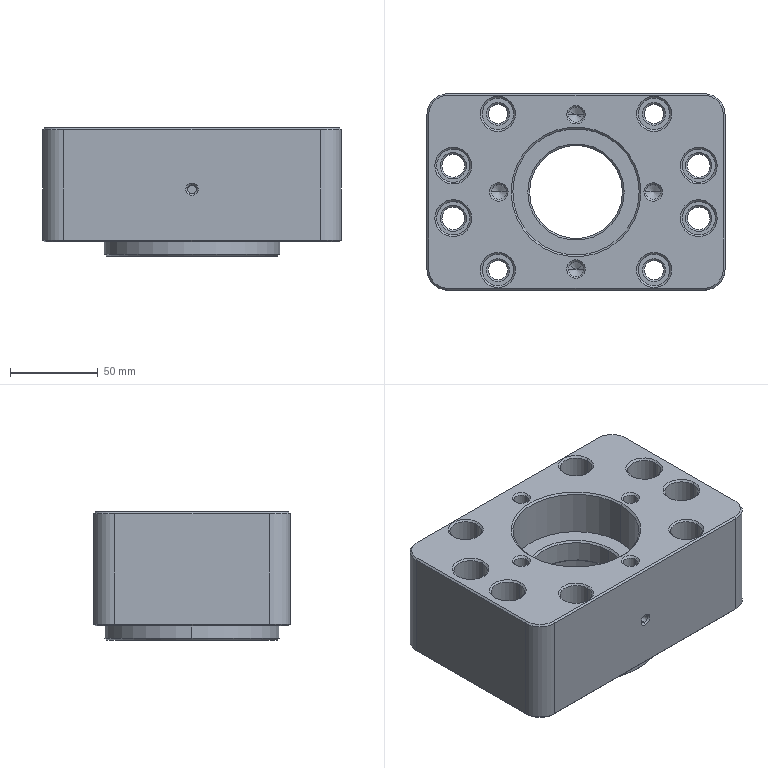Part | 1 solid | 199 faces | box 170 x 112 x 73 mm | volume 874233 mm3 | cone 106 | cylinder 66 | plane 25 | spline 2 | commonest cylinder face diameters 3.3 x8 8.5 x8 11 x8 13 x8 18 x8 19 x8